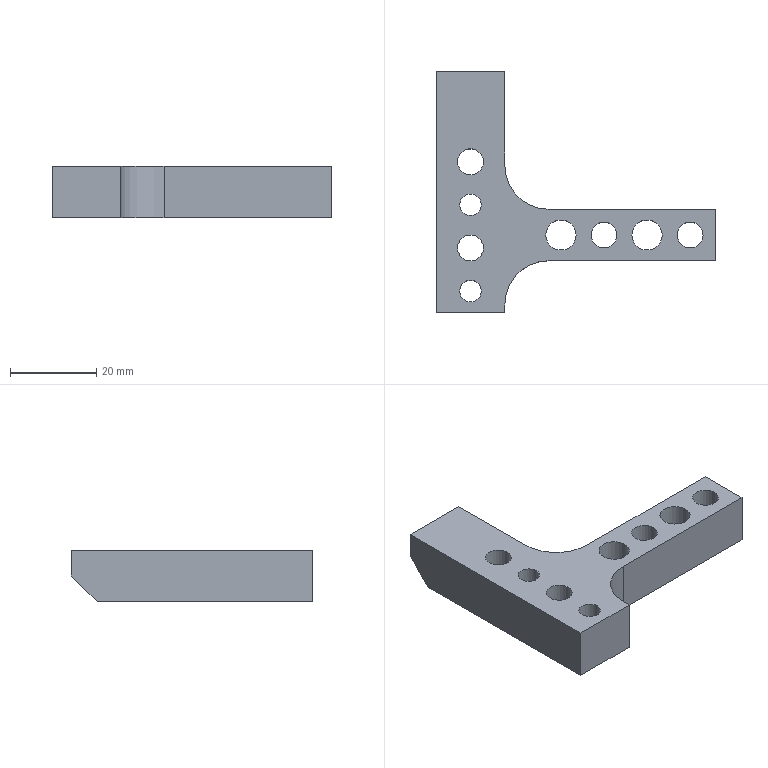Part | NX | features BREP 1 | 1 solid | 21 faces | box 65 x 56 x 12 mm | volume 15283 mm3 | plane 11 | cylinder 10 | commonest cylinder face diameters 6 x4 5 x2 7 x2 20 x2
STEP:
#1=CARTESIAN_POINT('',(26.,0.,-12.));
#2=VERTEX_POINT('',#1);
#3=CARTESIAN_POINT('',(65.,0.,-12.));
#4=VERTEX_POINT('',#3);
#5=CARTESIAN_POINT('',(0.,0.,-12.));
#6=DIRECTION('',(1.,0.,0.));
#7=VECTOR('',#6,1000.);
#8=LINE('',#5,#7);
#9=EDGE_CURVE('',#2,#4,#8,.T.);
#10=ORIENTED_EDGE('',*,*,#9,.T.);
#11=CARTESIAN_POINT('',(65.,0.,0.));
#12=VERTEX_POINT('',#11);
#13=CARTESIAN_POINT('',(65.,0.,-12.));
#14=DIRECTION('',(0.,0.,1.));
#15=VECTOR('',#14,1000.);
#16=LINE('',#13,#15);
#17=EDGE_CURVE('',#4,#12,#16,.T.);
#18=ORIENTED_EDGE('',*,*,#17,.T.);
#19=CARTESIAN_POINT('',(26.,0.,0.));
#20=VERTEX_POINT('',#19);
#21=CARTESIAN_POINT('',(0.,0.,0.));
#22=DIRECTION('',(1.,0.,0.));
#23=VECTOR('',#22,1000.);
#24=LINE('',#21,#23);
#25=EDGE_CURVE('',#20,#12,#24,.T.);
#26=ORIENTED_EDGE('',*,*,#25,.F.);
#27=CARTESIAN_POINT('',(26.,0.,-12.));
#28=DIRECTION('',(0.,0.,1.));
#29=VECTOR('',#28,1000.);
#30=LINE('',#27,#29);
#31=EDGE_CURVE('',#2,#20,#30,.T.);
#32=ORIENTED_EDGE('',*,*,#31,.F.);
#33=EDGE_LOOP('',(#10,#18,#26,#32));
#34=FACE_BOUND('',#33,.T.);
#35=CARTESIAN_POINT('',(0.,0.,-12.));
#36=DIRECTION('',(0.,1.,0.));
#37=DIRECTION('',(0.,0.,1.));
#38=AXIS2_PLACEMENT_3D('',#35,#36,#37);
#39=PLANE('',#38);
#40=ADVANCED_FACE('',(#34),#39,.F.);
#41=CARTESIAN_POINT('',(0.,44.,-6.));
#42=VERTEX_POINT('',#41);
#43=CARTESIAN_POINT('',(0.,44.,0.));
#44=VERTEX_POINT('',#43);
#45=CARTESIAN_POINT('',(0.,44.,-12.));
#46=DIRECTION('',(0.,0.,1.));
#47=VECTOR('',#46,1000.);
#48=LINE('',#45,#47);
#49=EDGE_CURVE('',#42,#44,#48,.T.);
#50=ORIENTED_EDGE('',*,*,#49,.T.);
#51=CARTESIAN_POINT('',(16.,44.,0.));
#52=VERTEX_POINT('',#51);
#53=CARTESIAN_POINT('',(16.,44.,0.));
#54=DIRECTION('',(-1.,0.,0.));
#55=VECTOR('',#54,1000.);
#56=LINE('',#53,#55);
#57=EDGE_CURVE('',#52,#44,#56,.T.);
#58=ORIENTED_EDGE('',*,*,#57,.F.);
#59=CARTESIAN_POINT('',(16.,44.,-6.));
#60=VERTEX_POINT('',#59);
#61=CARTESIAN_POINT('',(16.,44.,-12.));
#62=DIRECTION('',(0.,0.,1.));
#63=VECTOR('',#62,1000.);
#64=LINE('',#61,#63);
#65=EDGE_CURVE('',#60,#52,#64,.T.);
#66=ORIENTED_EDGE('',*,*,#65,.F.);
#67=CARTESIAN_POINT('',(16.,44.,-6.));
#68=DIRECTION('',(1.,0.,0.));
#69=VECTOR('',#68,1000.);
#70=LINE('',#67,#69);
#71=EDGE_CURVE('',#42,#60,#70,.T.);
#72=ORIENTED_EDGE('',*,*,#71,.F.);
#73=EDGE_LOOP('',(#50,#58,#66,#72));
#74=FACE_BOUND('',#73,.T.);
#75=CARTESIAN_POINT('',(16.,44.,-12.));
#76=DIRECTION('',(0.,-1.,0.));
#77=DIRECTION('',(0.,0.,-1.));
#78=AXIS2_PLACEMENT_3D('',#75,#76,#77);
#79=PLANE('',#78);
#80=ADVANCED_FACE('',(#74),#79,.F.);
#81=CARTESIAN_POINT('',(0.,38.,-12.));
#82=VERTEX_POINT('',#81);
#83=CARTESIAN_POINT('',(0.,-12.,-12.));
#84=VERTEX_POINT('',#83);
#85=CARTESIAN_POINT('',(0.,44.,-12.));
#86=DIRECTION('',(0.,-1.,0.));
#87=VECTOR('',#86,1000.);
#88=LINE('',#85,#87);
#89=EDGE_CURVE('',#82,#84,#88,.T.);
#90=ORIENTED_EDGE('',*,*,#89,.T.);
#91=CARTESIAN_POINT('',(0.,-12.,0.));
#92=VERTEX_POINT('',#91);
#93=CARTESIAN_POINT('',(0.,-12.,0.));
#94=DIRECTION('',(0.,0.,-1.));
#95=VECTOR('',#94,1000.);
#96=LINE('',#93,#95);
#97=EDGE_CURVE('',#92,#84,#96,.T.);
#98=ORIENTED_EDGE('',*,*,#97,.F.);
#99=CARTESIAN_POINT('',(0.,44.,0.));
#100=DIRECTION('',(0.,-1.,0.));
#101=VECTOR('',#100,1000.);
#102=LINE('',#99,#101);
#103=EDGE_CURVE('',#44,#92,#102,.T.);
#104=ORIENTED_EDGE('',*,*,#103,.F.);
#105=ORIENTED_EDGE('',*,*,#49,.F.);
#106=CARTESIAN_POINT('',(0.,38.,-12.));
#107=DIRECTION('',(0.,0.7071,0.7071));
#108=VECTOR('',#107,1000.);
#109=LINE('',#106,#108);
#110=EDGE_CURVE('',#82,#42,#109,.T.);
#111=ORIENTED_EDGE('',*,*,#110,.F.);
#112=EDGE_LOOP('',(#90,#98,#104,#105,#111));
#113=FACE_BOUND('',#112,.T.);
#114=CARTESIAN_POINT('',(0.,44.,-12.));
#115=DIRECTION('',(1.,0.,0.));
#116=DIRECTION('',(0.,-1.,0.));
#117=AXIS2_PLACEMENT_3D('',#114,#115,#116);
#118=PLANE('',#117);
#119=ADVANCED_FACE('',(#113),#118,.F.);
#120=CARTESIAN_POINT('',(65.,12.,0.));
#121=VERTEX_POINT('',#120);
#122=CARTESIAN_POINT('',(65.,0.,0.));
#123=DIRECTION('',(0.,1.,0.));
#124=VECTOR('',#123,1000.);
#125=LINE('',#122,#124);
#126=EDGE_CURVE('',#12,#121,#125,.T.);
#127=ORIENTED_EDGE('',*,*,#126,.F.);
#128=ORIENTED_EDGE('',*,*,#17,.F.);
#129=CARTESIAN_POINT('',(65.,12.,-12.));
#130=VERTEX_POINT('',#129);
#131=CARTESIAN_POINT('',(65.,0.,-12.));
#132=DIRECTION('',(0.,1.,0.));
#133=VECTOR('',#132,1000.);
#134=LINE('',#131,#133);
#135=EDGE_CURVE('',#4,#130,#134,.T.);
#136=ORIENTED_EDGE('',*,*,#135,.T.);
#137=CARTESIAN_POINT('',(65.,12.,-12.));
#138=DIRECTION('',(0.,0.,1.));
#139=VECTOR('',#138,1000.);
#140=LINE('',#137,#139);
#141=EDGE_CURVE('',#130,#121,#140,.T.);
#142=ORIENTED_EDGE('',*,*,#141,.T.);
#143=EDGE_LOOP('',(#127,#128,#136,#142));
#144=FACE_BOUND('',#143,.T.);
#145=CARTESIAN_POINT('',(65.,0.,-12.));
#146=DIRECTION('',(-1.,0.,0.));
#147=DIRECTION('',(0.,0.,1.));
#148=AXIS2_PLACEMENT_3D('',#145,#146,#147);
#149=PLANE('',#148);
#150=ADVANCED_FACE('',(#144),#149,.F.);
#151=CARTESIAN_POINT('',(26.,12.,0.));
#152=VERTEX_POINT('',#151);
#153=CARTESIAN_POINT('',(65.,12.,0.));
#154=DIRECTION('',(-1.,0.,0.));
#155=VECTOR('',#154,1000.);
#156=LINE('',#153,#155);
#157=EDGE_CURVE('',#121,#152,#156,.T.);
#158=ORIENTED_EDGE('',*,*,#157,.F.);
#159=ORIENTED_EDGE('',*,*,#141,.F.);
#160=CARTESIAN_POINT('',(26.,12.,-12.));
#161=VERTEX_POINT('',#160);
#162=CARTESIAN_POINT('',(65.,12.,-12.));
#163=DIRECTION('',(-1.,0.,0.));
#164=VECTOR('',#163,1000.);
#165=LINE('',#162,#164);
#166=EDGE_CURVE('',#130,#161,#165,.T.);
#167=ORIENTED_EDGE('',*,*,#166,.T.);
#168=CARTESIAN_POINT('',(26.,12.,-12.));
#169=DIRECTION('',(0.,0.,-1.));
#170=VECTOR('',#169,1000.);
#171=LINE('',#168,#170);
#172=EDGE_CURVE('',#152,#161,#171,.T.);
#173=ORIENTED_EDGE('',*,*,#172,.F.);
#174=EDGE_LOOP('',(#158,#159,#167,#173));
#175=FACE_BOUND('',#174,.T.);
#176=CARTESIAN_POINT('',(65.,12.,-12.));
#177=DIRECTION('',(0.,-1.,0.));
#178=DIRECTION('',(-1.,0.,0.));
#179=AXIS2_PLACEMENT_3D('',#176,#177,#178);
#180=PLANE('',#179);
#181=ADVANCED_FACE('',(#175),#180,.F.);
#182=CARTESIAN_POINT('',(16.,22.,-12.));
#183=VERTEX_POINT('',#182);
#184=CARTESIAN_POINT('',(16.,38.,-12.));
#185=VERTEX_POINT('',#184);
#186=CARTESIAN_POINT('',(16.,12.,-12.));
#187=DIRECTION('',(0.,1.,0.));
#188=VECTOR('',#187,1000.);
#189=LINE('',#186,#188);
#190=EDGE_CURVE('',#183,#185,#189,.T.);
#191=ORIENTED_EDGE('',*,*,#190,.T.);
#192=CARTESIAN_POINT('',(16.,38.,-12.));
#193=DIRECTION('',(0.,-0.7071,-0.7071));
#194=VECTOR('',#193,1000.);
#195=LINE('',#192,#194);
#196=EDGE_CURVE('',#60,#185,#195,.T.);
#197=ORIENTED_EDGE('',*,*,#196,.F.);
#198=ORIENTED_EDGE('',*,*,#65,.T.);
#199=CARTESIAN_POINT('',(16.,22.,0.));
#200=VERTEX_POINT('',#199);
#201=CARTESIAN_POINT('',(16.,12.,0.));
#202=DIRECTION('',(0.,1.,0.));
#203=VECTOR('',#202,1000.);
#204=LINE('',#201,#203);
#205=EDGE_CURVE('',#200,#52,#204,.T.);
#206=ORIENTED_EDGE('',*,*,#205,.F.);
#207=CARTESIAN_POINT('',(16.,22.,0.));
#208=DIRECTION('',(0.,0.,1.));
#209=VECTOR('',#208,1000.);
#210=LINE('',#207,#209);
#211=EDGE_CURVE('',#183,#200,#210,.T.);
#212=ORIENTED_EDGE('',*,*,#211,.F.);
#213=EDGE_LOOP('',(#191,#197,#198,#206,#212));
#214=FACE_BOUND('',#213,.T.);
#215=CARTESIAN_POINT('',(16.,12.,-12.));
#216=DIRECTION('',(-1.,0.,0.));
#217=DIRECTION('',(0.,0.,1.));
#218=AXIS2_PLACEMENT_3D('',#215,#216,#217);
#219=PLANE('',#218);
#220=ADVANCED_FACE('',(#214),#219,.F.);
#221=CARTESIAN_POINT('',(52.5,6.,-12.));
#222=VERTEX_POINT('',#221);
#223=CARTESIAN_POINT('',(49.,6.,-12.));
#224=DIRECTION('',(0.,0.,1.));
#225=DIRECTION('',(1.,0.,0.));
#226=AXIS2_PLACEMENT_3D('',#223,#224,#225);
#227=CIRCLE('',#226,3.5);
#228=EDGE_CURVE('',#222,#222,#227,.T.);
#229=ORIENTED_EDGE('',*,*,#228,.T.);
#230=EDGE_LOOP('',(#229));
#231=FACE_BOUND('',#230,.T.);
#232=CARTESIAN_POINT('',(32.5,6.,-12.));
#233=VERTEX_POINT('',#232);
#234=CARTESIAN_POINT('',(29.,6.,-12.));
#235=DIRECTION('',(0.,0.,1.));
#236=DIRECTION('',(1.,0.,0.));
#237=AXIS2_PLACEMENT_3D('',#234,#235,#236);
#238=CIRCLE('',#237,3.5);
#239=EDGE_CURVE('',#233,#233,#238,.T.);
#240=ORIENTED_EDGE('',*,*,#239,.T.);
#241=EDGE_LOOP('',(#240));
#242=FACE_BOUND('',#241,.T.);
#243=CARTESIAN_POINT('',(62.,6.,-12.));
#244=VERTEX_POINT('',#243);
#245=CARTESIAN_POINT('',(59.,6.,-12.));
#246=DIRECTION('',(0.,0.,1.));
#247=DIRECTION('',(1.,0.,0.));
#248=AXIS2_PLACEMENT_3D('',#245,#246,#247);
#249=CIRCLE('',#248,3.);
#250=EDGE_CURVE('',#244,#244,#249,.T.);
#251=ORIENTED_EDGE('',*,*,#250,.T.);
#252=EDGE_LOOP('',(#251));
#253=FACE_BOUND('',#252,.T.);
#254=CARTESIAN_POINT('',(42.,6.,-12.));
#255=VERTEX_POINT('',#254);
#256=CARTESIAN_POINT('',(39.,6.,-12.));
#257=DIRECTION('',(0.,0.,1.));
#258=DIRECTION('',(1.,0.,0.));
#259=AXIS2_PLACEMENT_3D('',#256,#257,#258);
#260=CIRCLE('',#259,3.);
#261=EDGE_CURVE('',#255,#255,#260,.T.);
#262=ORIENTED_EDGE('',*,*,#261,.T.);
#263=EDGE_LOOP('',(#262));
#264=FACE_BOUND('',#263,.T.);
#265=CARTESIAN_POINT('',(5.,3.,-12.));
#266=VERTEX_POINT('',#265);
#267=CARTESIAN_POINT('',(8.,3.,-12.));
#268=DIRECTION('',(0.,0.,-1.));
#269=DIRECTION('',(-1.,0.,0.));
#270=AXIS2_PLACEMENT_3D('',#267,#268,#269);
#271=CIRCLE('',#270,3.);
#272=EDGE_CURVE('',#266,#266,#271,.T.);
#273=ORIENTED_EDGE('',*,*,#272,.F.);
#274=EDGE_LOOP('',(#273));
#275=FACE_BOUND('',#274,.T.);
#276=CARTESIAN_POINT('',(5.,23.,-12.));
#277=VERTEX_POINT('',#276);
#278=CARTESIAN_POINT('',(8.,23.,-12.));
#279=DIRECTION('',(0.,0.,-1.));
#280=DIRECTION('',(-1.,0.,0.));
#281=AXIS2_PLACEMENT_3D('',#278,#279,#280);
#282=CIRCLE('',#281,3.);
#283=EDGE_CURVE('',#277,#277,#282,.T.);
#284=ORIENTED_EDGE('',*,*,#283,.F.);
#285=EDGE_LOOP('',(#284));
#286=FACE_BOUND('',#285,.T.);
#287=CARTESIAN_POINT('',(5.5,-7.,-12.));
#288=VERTEX_POINT('',#287);
#289=CARTESIAN_POINT('',(8.,-7.,-12.));
#290=DIRECTION('',(0.,0.,-1.));
#291=DIRECTION('',(-1.,0.,0.));
#292=AXIS2_PLACEMENT_3D('',#289,#290,#291);
#293=CIRCLE('',#292,2.5);
#294=EDGE_CURVE('',#288,#288,#293,.T.);
#295=ORIENTED_EDGE('',*,*,#294,.F.);
#296=EDGE_LOOP('',(#295));
#297=FACE_BOUND('',#296,.T.);
#298=CARTESIAN_POINT('',(5.5,13.,-12.));
#299=VERTEX_POINT('',#298);
#300=CARTESIAN_POINT('',(8.,13.,-12.));
#301=DIRECTION('',(0.,0.,-1.));
#302=DIRECTION('',(-1.,0.,0.));
#303=AXIS2_PLACEMENT_3D('',#300,#301,#302);
#304=CIRCLE('',#303,2.5);
#305=EDGE_CURVE('',#299,#299,#304,.T.);
#306=ORIENTED_EDGE('',*,*,#305,.F.);
#307=EDGE_LOOP('',(#306));
#308=FACE_BOUND('',#307,.T.);
#309=ORIENTED_EDGE('',*,*,#166,.F.);
#310=ORIENTED_EDGE('',*,*,#135,.F.);
#311=ORIENTED_EDGE('',*,*,#9,.F.);
#312=CARTESIAN_POINT('',(16.,-10.,-12.));
#313=VERTEX_POINT('',#312);
#314=CARTESIAN_POINT('',(26.,-10.,-12.));
#315=DIRECTION('',(0.,0.,-1.));
#316=DIRECTION('',(1.,0.,0.));
#317=AXIS2_PLACEMENT_3D('',#314,#315,#316);
#318=CIRCLE('',#317,10.);
#319=EDGE_CURVE('',#313,#2,#318,.T.);
#320=ORIENTED_EDGE('',*,*,#319,.F.);
#321=CARTESIAN_POINT('',(16.,-12.,-12.));
#322=VERTEX_POINT('',#321);
#323=CARTESIAN_POINT('',(16.,-12.,-12.));
#324=DIRECTION('',(0.,1.,0.));
#325=VECTOR('',#324,1000.);
#326=LINE('',#323,#325);
#327=EDGE_CURVE('',#322,#313,#326,.T.);
#328=ORIENTED_EDGE('',*,*,#327,.F.);
#329=CARTESIAN_POINT('',(16.,-12.,-12.));
#330=DIRECTION('',(1.,0.,0.));
#331=VECTOR('',#330,1000.);
#332=LINE('',#329,#331);
#333=EDGE_CURVE('',#84,#322,#332,.T.);
#334=ORIENTED_EDGE('',*,*,#333,.F.);
#335=ORIENTED_EDGE('',*,*,#89,.F.);
#336=CARTESIAN_POINT('',(0.,38.,-12.));
#337=DIRECTION('',(-1.,0.,0.));
#338=VECTOR('',#337,1000.);
#339=LINE('',#336,#338);
#340=EDGE_CURVE('',#185,#82,#339,.T.);
#341=ORIENTED_EDGE('',*,*,#340,.F.);
#342=ORIENTED_EDGE('',*,*,#190,.F.);
#343=CARTESIAN_POINT('',(26.,22.,-12.));
#344=DIRECTION('',(0.,0.,-1.));
#345=DIRECTION('',(1.,0.,0.));
#346=AXIS2_PLACEMENT_3D('',#343,#344,#345);
#347=CIRCLE('',#346,10.);
#348=EDGE_CURVE('',#161,#183,#347,.T.);
#349=ORIENTED_EDGE('',*,*,#348,.F.);
#350=EDGE_LOOP('',(#309,#310,#311,#320,#328,#334,#335,#341,#342,#349));
#351=FACE_BOUND('',#350,.T.);
#352=CARTESIAN_POINT('',(0.,0.,-12.));
#353=DIRECTION('',(0.,0.,-1.));
#354=DIRECTION('',(-1.,0.,0.));
#355=AXIS2_PLACEMENT_3D('',#352,#353,#354);
#356=PLANE('',#355);
#357=ADVANCED_FACE('',(#231,#242,#253,#264,#275,#286,#297,#308,#351),#356,.T.);
#358=CARTESIAN_POINT('',(52.5,6.,0.));
#359=VERTEX_POINT('',#358);
#360=CARTESIAN_POINT('',(49.,6.,0.));
#361=DIRECTION('',(0.,0.,1.));
#362=DIRECTION('',(1.,0.,0.));
#363=AXIS2_PLACEMENT_3D('',#360,#361,#362);
#364=CIRCLE('',#363,3.5);
#365=EDGE_CURVE('',#359,#359,#364,.T.);
#366=ORIENTED_EDGE('',*,*,#365,.F.);
#367=EDGE_LOOP('',(#366));
#368=FACE_BOUND('',#367,.T.);
#369=CARTESIAN_POINT('',(32.5,6.,0.));
#370=VERTEX_POINT('',#369);
#371=CARTESIAN_POINT('',(29.,6.,0.));
#372=DIRECTION('',(0.,0.,1.));
#373=DIRECTION('',(1.,0.,0.));
#374=AXIS2_PLACEMENT_3D('',#371,#372,#373);
#375=CIRCLE('',#374,3.5);
#376=EDGE_CURVE('',#370,#370,#375,.T.);
#377=ORIENTED_EDGE('',*,*,#376,.F.);
#378=EDGE_LOOP('',(#377));
#379=FACE_BOUND('',#378,.T.);
#380=CARTESIAN_POINT('',(62.,6.,0.));
#381=VERTEX_POINT('',#380);
#382=CARTESIAN_POINT('',(59.,6.,0.));
#383=DIRECTION('',(0.,0.,1.));
#384=DIRECTION('',(1.,0.,0.));
#385=AXIS2_PLACEMENT_3D('',#382,#383,#384);
#386=CIRCLE('',#385,3.);
#387=EDGE_CURVE('',#381,#381,#386,.T.);
#388=ORIENTED_EDGE('',*,*,#387,.F.);
#389=EDGE_LOOP('',(#388));
#390=FACE_BOUND('',#389,.T.);
#391=CARTESIAN_POINT('',(42.,6.,0.));
#392=VERTEX_POINT('',#391);
#393=CARTESIAN_POINT('',(39.,6.,0.));
#394=DIRECTION('',(0.,0.,1.));
#395=DIRECTION('',(1.,0.,0.));
#396=AXIS2_PLACEMENT_3D('',#393,#394,#395);
#397=CIRCLE('',#396,3.);
#398=EDGE_CURVE('',#392,#392,#397,.T.);
#399=ORIENTED_EDGE('',*,*,#398,.F.);
#400=EDGE_LOOP('',(#399));
#401=FACE_BOUND('',#400,.T.);
#402=CARTESIAN_POINT('',(5.,3.,0.));
#403=VERTEX_POINT('',#402);
#404=CARTESIAN_POINT('',(8.,3.,0.));
#405=DIRECTION('',(0.,0.,-1.));
#406=DIRECTION('',(-1.,0.,0.));
#407=AXIS2_PLACEMENT_3D('',#404,#405,#406);
#408=CIRCLE('',#407,3.);
#409=EDGE_CURVE('',#403,#403,#408,.T.);
#410=ORIENTED_EDGE('',*,*,#409,.T.);
#411=EDGE_LOOP('',(#410));
#412=FACE_BOUND('',#411,.T.);
#413=CARTESIAN_POINT('',(5.,23.,0.));
#414=VERTEX_POINT('',#413);
#415=CARTESIAN_POINT('',(8.,23.,0.));
#416=DIRECTION('',(0.,0.,-1.));
#417=DIRECTION('',(-1.,0.,0.));
#418=AXIS2_PLACEMENT_3D('',#415,#416,#417);
#419=CIRCLE('',#418,3.);
#420=EDGE_CURVE('',#414,#414,#419,.T.);
#421=ORIENTED_EDGE('',*,*,#420,.T.);
#422=EDGE_LOOP('',(#421));
#423=FACE_BOUND('',#422,.T.);
#424=CARTESIAN_POINT('',(5.5,-7.,0.));
#425=VERTEX_POINT('',#424);
#426=CARTESIAN_POINT('',(8.,-7.,0.));
#427=DIRECTION('',(0.,0.,-1.));
#428=DIRECTION('',(-1.,0.,0.));
#429=AXIS2_PLACEMENT_3D('',#426,#427,#428);
#430=CIRCLE('',#429,2.5);
#431=EDGE_CURVE('',#425,#425,#430,.T.);
#432=ORIENTED_EDGE('',*,*,#431,.T.);
#433=EDGE_LOOP('',(#432));
#434=FACE_BOUND('',#433,.T.);
#435=CARTESIAN_POINT('',(5.5,13.,0.));
#436=VERTEX_POINT('',#435);
#437=CARTESIAN_POINT('',(8.,13.,0.));
#438=DIRECTION('',(0.,0.,-1.));
#439=DIRECTION('',(-1.,0.,0.));
#440=AXIS2_PLACEMENT_3D('',#437,#438,#439);
#441=CIRCLE('',#440,2.5);
#442=EDGE_CURVE('',#436,#436,#441,.T.);
#443=ORIENTED_EDGE('',*,*,#442,.T.);
#444=EDGE_LOOP('',(#443));
#445=FACE_BOUND('',#444,.T.);
#446=ORIENTED_EDGE('',*,*,#57,.T.);
#447=ORIENTED_EDGE('',*,*,#103,.T.);
#448=CARTESIAN_POINT('',(16.,-12.,0.));
#449=VERTEX_POINT('',#448);
#450=CARTESIAN_POINT('',(16.,-12.,0.));
#451=DIRECTION('',(1.,0.,0.));
#452=VECTOR('',#451,1000.);
#453=LINE('',#450,#452);
#454=EDGE_CURVE('',#92,#449,#453,.T.);
#455=ORIENTED_EDGE('',*,*,#454,.T.);
#456=CARTESIAN_POINT('',(16.,-10.,0.));
#457=VERTEX_POINT('',#456);
#458=CARTESIAN_POINT('',(16.,-12.,0.));
#459=DIRECTION('',(0.,1.,0.));
#460=VECTOR('',#459,1000.);
#461=LINE('',#458,#460);
#462=EDGE_CURVE('',#449,#457,#461,.T.);
#463=ORIENTED_EDGE('',*,*,#462,.T.);
#464=CARTESIAN_POINT('',(26.,-10.,0.));
#465=DIRECTION('',(0.,0.,1.));
#466=DIRECTION('',(1.,0.,0.));
#467=AXIS2_PLACEMENT_3D('',#464,#465,#466);
#468=CIRCLE('',#467,10.);
#469=EDGE_CURVE('',#20,#457,#468,.T.);
#470=ORIENTED_EDGE('',*,*,#469,.F.);
#471=ORIENTED_EDGE('',*,*,#25,.T.);
#472=ORIENTED_EDGE('',*,*,#126,.T.);
#473=ORIENTED_EDGE('',*,*,#157,.T.);
#474=CARTESIAN_POINT('',(26.,22.,0.));
#475=DIRECTION('',(0.,0.,1.));
#476=DIRECTION('',(1.,0.,0.));
#477=AXIS2_PLACEMENT_3D('',#474,#475,#476);
#478=CIRCLE('',#477,10.);
#479=EDGE_CURVE('',#200,#152,#478,.T.);
#480=ORIENTED_EDGE('',*,*,#479,.F.);
#481=ORIENTED_EDGE('',*,*,#205,.T.);
#482=EDGE_LOOP('',(#446,#447,#455,#463,#470,#471,#472,#473,#480,#481));
#483=FACE_BOUND('',#482,.T.);
#484=CARTESIAN_POINT('',(0.,0.,0.));
#485=DIRECTION('',(0.,0.,-1.));
#486=DIRECTION('',(-1.,0.,0.));
#487=AXIS2_PLACEMENT_3D('',#484,#485,#486);
#488=PLANE('',#487);
#489=ADVANCED_FACE('',(#368,#379,#390,#401,#412,#423,#434,#445,#483),#488,.F.);
#490=ORIENTED_EDGE('',*,*,#196,.T.);
#491=ORIENTED_EDGE('',*,*,#340,.T.);
#492=ORIENTED_EDGE('',*,*,#110,.T.);
#493=ORIENTED_EDGE('',*,*,#71,.T.);
#494=EDGE_LOOP('',(#490,#491,#492,#493));
#495=FACE_BOUND('',#494,.T.);
#496=CARTESIAN_POINT('',(0.,38.,-12.));
#497=DIRECTION('',(0.,0.7071,-0.7071));
#498=DIRECTION('',(-1.,0.,0.));
#499=AXIS2_PLACEMENT_3D('',#496,#497,#498);
#500=PLANE('',#499);
#501=ADVANCED_FACE('',(#495),#500,.T.);
#502=ORIENTED_EDGE('',*,*,#462,.F.);
#503=CARTESIAN_POINT('',(16.,-12.,0.));
#504=DIRECTION('',(0.,0.,-1.));
#505=VECTOR('',#504,1000.);
#506=LINE('',#503,#505);
#507=EDGE_CURVE('',#449,#322,#506,.T.);
#508=ORIENTED_EDGE('',*,*,#507,.T.);
#509=ORIENTED_EDGE('',*,*,#327,.T.);
#510=CARTESIAN_POINT('',(16.,-10.,0.));
#511=DIRECTION('',(0.,0.,-1.));
#512=VECTOR('',#511,1000.);
#513=LINE('',#510,#512);
#514=EDGE_CURVE('',#457,#313,#513,.T.);
#515=ORIENTED_EDGE('',*,*,#514,.F.);
#516=EDGE_LOOP('',(#502,#508,#509,#515));
#517=FACE_BOUND('',#516,.T.);
#518=CARTESIAN_POINT('',(16.,-12.,0.));
#519=DIRECTION('',(1.,0.,0.));
#520=DIRECTION('',(0.,0.,-1.));
#521=AXIS2_PLACEMENT_3D('',#518,#519,#520);
#522=PLANE('',#521);
#523=ADVANCED_FACE('',(#517),#522,.T.);
#524=ORIENTED_EDGE('',*,*,#333,.T.);
#525=ORIENTED_EDGE('',*,*,#507,.F.);
#526=ORIENTED_EDGE('',*,*,#454,.F.);
#527=ORIENTED_EDGE('',*,*,#97,.T.);
#528=EDGE_LOOP('',(#524,#525,#526,#527));
#529=FACE_BOUND('',#528,.T.);
#530=CARTESIAN_POINT('',(16.,-12.,0.));
#531=DIRECTION('',(0.,-1.,0.));
#532=DIRECTION('',(-1.,0.,0.));
#533=AXIS2_PLACEMENT_3D('',#530,#531,#532);
#534=PLANE('',#533);
#535=ADVANCED_FACE('',(#529),#534,.T.);
#536=ORIENTED_EDGE('',*,*,#469,.T.);
#537=ORIENTED_EDGE('',*,*,#514,.T.);
#538=ORIENTED_EDGE('',*,*,#319,.T.);
#539=ORIENTED_EDGE('',*,*,#31,.T.);
#540=EDGE_LOOP('',(#536,#537,#538,#539));
#541=FACE_BOUND('',#540,.T.);
#542=CARTESIAN_POINT('',(26.,-10.,0.));
#543=DIRECTION('',(0.,0.,-1.));
#544=DIRECTION('',(-1.,0.,0.));
#545=AXIS2_PLACEMENT_3D('',#542,#543,#544);
#546=CYLINDRICAL_SURFACE('',#545,10.);
#547=ADVANCED_FACE('',(#541),#546,.F.);
#548=ORIENTED_EDGE('',*,*,#348,.T.);
#549=ORIENTED_EDGE('',*,*,#211,.T.);
#550=ORIENTED_EDGE('',*,*,#479,.T.);
#551=ORIENTED_EDGE('',*,*,#172,.T.);
#552=EDGE_LOOP('',(#548,#549,#550,#551));
#553=FACE_BOUND('',#552,.T.);
#554=CARTESIAN_POINT('',(26.,22.,-12.));
#555=DIRECTION('',(0.,0.,-1.));
#556=DIRECTION('',(-1.,0.,0.));
#557=AXIS2_PLACEMENT_3D('',#554,#555,#556);
#558=CYLINDRICAL_SURFACE('',#557,10.);
#559=ADVANCED_FACE('',(#553),#558,.F.);
#560=ORIENTED_EDGE('',*,*,#305,.T.);
#561=EDGE_LOOP('',(#560));
#562=FACE_BOUND('',#561,.T.);
#563=ORIENTED_EDGE('',*,*,#442,.F.);
#564=EDGE_LOOP('',(#563));
#565=FACE_BOUND('',#564,.T.);
#566=CARTESIAN_POINT('',(8.,13.,0.));
#567=DIRECTION('',(0.,0.,1.));
#568=DIRECTION('',(1.,0.,0.));
#569=AXIS2_PLACEMENT_3D('',#566,#567,#568);
#570=CYLINDRICAL_SURFACE('',#569,2.5);
#571=ADVANCED_FACE('',(#562,#565),#570,.F.);
#572=ORIENTED_EDGE('',*,*,#294,.T.);
#573=EDGE_LOOP('',(#572));
#574=FACE_BOUND('',#573,.T.);
#575=ORIENTED_EDGE('',*,*,#431,.F.);
#576=EDGE_LOOP('',(#575));
#577=FACE_BOUND('',#576,.T.);
#578=CARTESIAN_POINT('',(8.,-7.,0.));
#579=DIRECTION('',(0.,0.,1.));
#580=DIRECTION('',(1.,0.,0.));
#581=AXIS2_PLACEMENT_3D('',#578,#579,#580);
#582=CYLINDRICAL_SURFACE('',#581,2.5);
#583=ADVANCED_FACE('',(#574,#577),#582,.F.);
#584=ORIENTED_EDGE('',*,*,#283,.T.);
#585=EDGE_LOOP('',(#584));
#586=FACE_BOUND('',#585,.T.);
#587=ORIENTED_EDGE('',*,*,#420,.F.);
#588=EDGE_LOOP('',(#587));
#589=FACE_BOUND('',#588,.T.);
#590=CARTESIAN_POINT('',(8.,23.,0.));
#591=DIRECTION('',(0.,0.,1.));
#592=DIRECTION('',(1.,0.,0.));
#593=AXIS2_PLACEMENT_3D('',#590,#591,#592);
#594=CYLINDRICAL_SURFACE('',#593,3.);
#595=ADVANCED_FACE('',(#586,#589),#594,.F.);
#596=ORIENTED_EDGE('',*,*,#272,.T.);
#597=EDGE_LOOP('',(#596));
#598=FACE_BOUND('',#597,.T.);
#599=ORIENTED_EDGE('',*,*,#409,.F.);
#600=EDGE_LOOP('',(#599));
#601=FACE_BOUND('',#600,.T.);
#602=CARTESIAN_POINT('',(8.,3.,0.));
#603=DIRECTION('',(0.,0.,1.));
#604=DIRECTION('',(1.,0.,0.));
#605=AXIS2_PLACEMENT_3D('',#602,#603,#604);
#606=CYLINDRICAL_SURFACE('',#605,3.);
#607=ADVANCED_FACE('',(#598,#601),#606,.F.);
#608=ORIENTED_EDGE('',*,*,#398,.T.);
#609=EDGE_LOOP('',(#608));
#610=FACE_BOUND('',#609,.T.);
#611=ORIENTED_EDGE('',*,*,#261,.F.);
#612=EDGE_LOOP('',(#611));
#613=FACE_BOUND('',#612,.T.);
#614=CARTESIAN_POINT('',(39.,6.,-12.));
#615=DIRECTION('',(0.,0.,-1.));
#616=DIRECTION('',(-1.,0.,0.));
#617=AXIS2_PLACEMENT_3D('',#614,#615,#616);
#618=CYLINDRICAL_SURFACE('',#617,3.);
#619=ADVANCED_FACE('',(#610,#613),#618,.F.);
#620=ORIENTED_EDGE('',*,*,#387,.T.);
#621=EDGE_LOOP('',(#620));
#622=FACE_BOUND('',#621,.T.);
#623=ORIENTED_EDGE('',*,*,#250,.F.);
#624=EDGE_LOOP('',(#623));
#625=FACE_BOUND('',#624,.T.);
#626=CARTESIAN_POINT('',(59.,6.,-12.));
#627=DIRECTION('',(0.,0.,-1.));
#628=DIRECTION('',(-1.,0.,0.));
#629=AXIS2_PLACEMENT_3D('',#626,#627,#628);
#630=CYLINDRICAL_SURFACE('',#629,3.);
#631=ADVANCED_FACE('',(#622,#625),#630,.F.);
#632=ORIENTED_EDGE('',*,*,#376,.T.);
#633=EDGE_LOOP('',(#632));
#634=FACE_BOUND('',#633,.T.);
#635=ORIENTED_EDGE('',*,*,#239,.F.);
#636=EDGE_LOOP('',(#635));
#637=FACE_BOUND('',#636,.T.);
#638=CARTESIAN_POINT('',(29.,6.,-12.));
#639=DIRECTION('',(0.,0.,-1.));
#640=DIRECTION('',(-1.,0.,0.));
#641=AXIS2_PLACEMENT_3D('',#638,#639,#640);
#642=CYLINDRICAL_SURFACE('',#641,3.5);
#643=ADVANCED_FACE('',(#634,#637),#642,.F.);
#644=ORIENTED_EDGE('',*,*,#365,.T.);
#645=EDGE_LOOP('',(#644));
#646=FACE_BOUND('',#645,.T.);
#647=ORIENTED_EDGE('',*,*,#228,.F.);
#648=EDGE_LOOP('',(#647));
#649=FACE_BOUND('',#648,.T.);
#650=CARTESIAN_POINT('',(49.,6.,-12.));
#651=DIRECTION('',(0.,0.,-1.));
#652=DIRECTION('',(-1.,0.,0.));
#653=AXIS2_PLACEMENT_3D('',#650,#651,#652);
#654=CYLINDRICAL_SURFACE('',#653,3.5);
#655=ADVANCED_FACE('',(#646,#649),#654,.F.);
#656=CLOSED_SHELL('',(#40,#80,#119,#150,#181,#220,#357,#489,#501,#523,#535,#547,#559,#571,#583,#595,#607,#619,#631,#643,#655));
#657=MANIFOLD_SOLID_BREP('',#656);
#658=(LENGTH_UNIT()NAMED_UNIT(*)SI_UNIT(.MILLI.,.METRE.));
#659=UNCERTAINTY_MEASURE_WITH_UNIT(LENGTH_MEASURE(0.00001),#658,'','');
#660=(NAMED_UNIT(*)PLANE_ANGLE_UNIT()SI_UNIT($,.RADIAN.));
#661=(NAMED_UNIT(*)SI_UNIT($,.STERADIAN.)SOLID_ANGLE_UNIT());
#662=(GEOMETRIC_REPRESENTATION_CONTEXT(3)GLOBAL_UNCERTAINTY_ASSIGNED_CONTEXT((#659))GLOBAL_UNIT_ASSIGNED_CONTEXT((#658,#660,#661))REPRESENTATION_CONTEXT('',''));
#663=ADVANCED_BREP_SHAPE_REPRESENTATION('',(#657),#662);